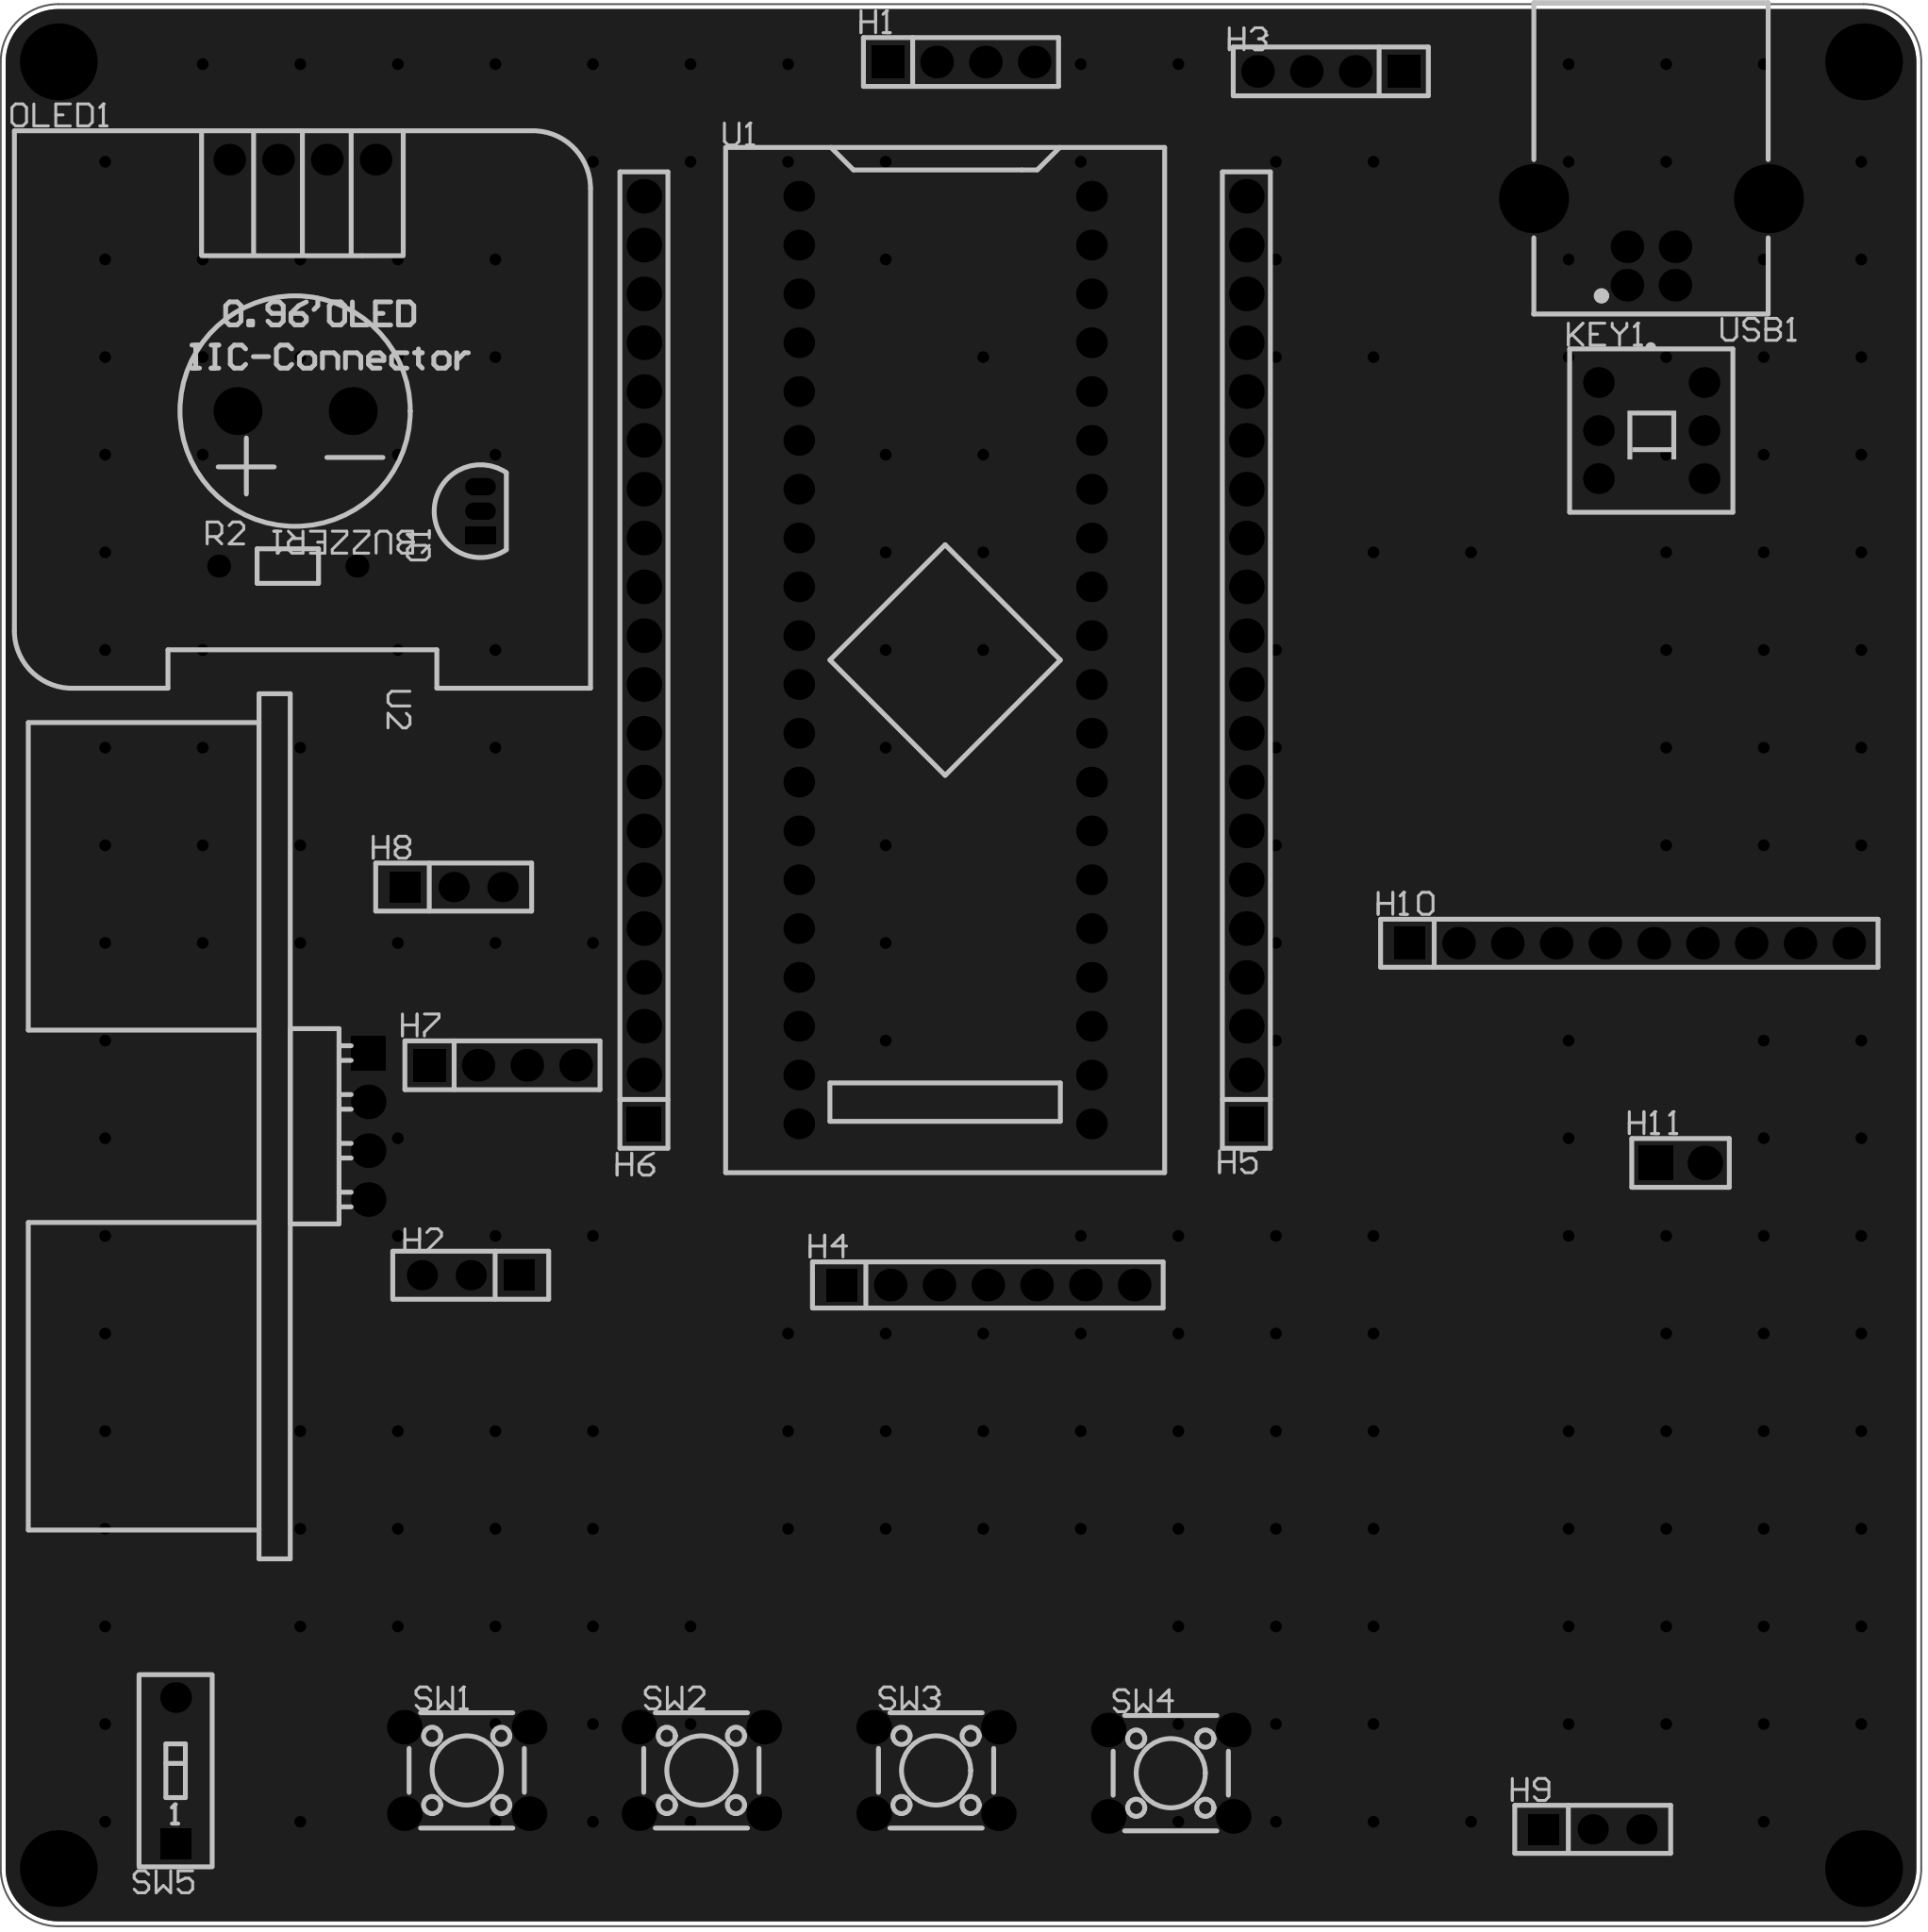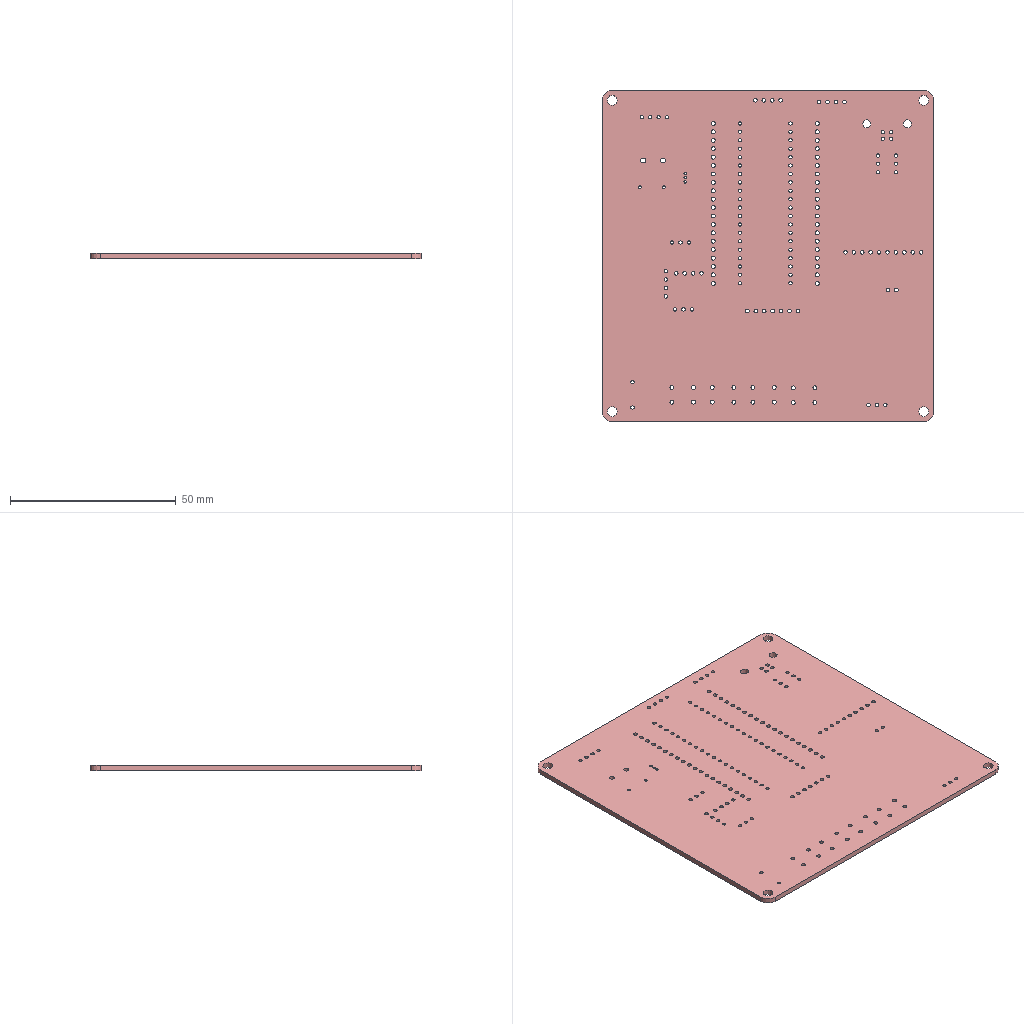Circuit board layout | Altium Designer | box 100 x 100 x 1.6 mm
Layer stack:
# Altium Designer layer stack of  (unit mm; dielectric type: 0 none, 1 core, 2 prepreg, 3 surface material)
index,name,kind,layer,copper_thickness_mm,dielectric_type,dielectric_thickness_mm,dielectric_material,dielectric_constant
0,Top Paste Mask Layer,other,,,,,,
1,Top Silkscreen Layer,other,,,,,,
2,Top Solder Mask Layer,dielectric,,,3,0.01,,3.3
3,Top Layer,copper,Top Layer,0.035,,,,
4,Dielectric1,dielectric,,,3,1.51,FR4,4.5
5,Bottom Layer,copper,Bottom Layer,0.035,,,,
6,Bottom Solder Mask Layer,dielectric,,,3,0.01,,3.3
7,Bottom Silkscreen Layer,other,,,,,,
8,Bottom Paste Mask Layer,other,,,,,,
# drill layer pairs: low layer,high layer
drill_pair,Top Layer,Bottom Layer
Part placement:
Designator,Comment,Layer,Footprint,Center-X(mm),Center-Y(mm),Rotation
BUZZER1,buzzer,TopLayer,BUZ-TH_BD12.0-P6.00-D0.9-RD,95.885,157.734,180
H1,,TopLayer,HDR-TH_4P-P2.54-V-M,130.556,175.895,0
H2,,TopLayer,HDR-TH_3P-P2.54-V-F,105.029,112.776,180
H3,,TopLayer,HDR-TH_4P-P2.54-V-M,149.81,175.405,180
H4,,TopLayer,HDR-TH_7P-P2.54-V-F,131.953,112.268,0
H5,,TopLayer,HDR-TH_20P-P2.54-V-M-1,145.415,144.78,90
H6,,TopLayer,HDR-TH_20P-P2.54-V-M-1,114.046,144.78,90
H7,,TopLayer,HDR-TH_4P-P2.54-V-M,106.68,123.698,0
H8,,TopLayer,HDR-TH_3P-P2.54-V-F,104.14,132.969,0
H9,,TopLayer,HDR-TH_3P-P2.54-V-F,163.449,83.947,0
H10,,TopLayer,HDR-TH_10P-P2.54-V-F,165.354,130.048,0
H11,,TopLayer,HDR-TH_2P-P2.54-V-M-1,168.021,118.618,0
KEY1,Non-latching switch 8.5×8.5, silent,TopLayer,SW-TH_6P-L8.5-W8.5-P2.54,166.497,156.718,270
OLED1,,TopLayer,0.96OLED_4P,96.266,170.815,0
Q1,,TopLayer,S8050_TO_92,105.537,152.527,90
R2,10kΩ,TopLayer,Res_1/8W,95.504,149.669,0
SW5,NDS-01V,TopLayer,SW-TH_2P-L3.9-W9.9-P2.54-LS7.6,89.662,86.995,90
U1,STM32F103C8T6-Card,TopLayer,CONN-TH_L53.3-W22.9_STM32F103C8T6-CARD,129.731,144.78,270
U2,HC-SR04,TopLayer,TH_HC-SR04V,99.695,120.523,270
USB1,,TopLayer,USB__Type-B,166.484,166.533,180
SW1,,TopLayer,SW-TH_4P-L6.0-W6.0-P4.50-LS6.5,104.819,87.011,180
SW2,,TopLayer,SW-TH_4P-L6.0-W6.0-P4.50-LS6.5,117.038,87.011,180
SW3,,TopLayer,SW-TH_4P-L6.0-W6.0-P4.50-LS6.5,129.258,87.011,180
SW4,,TopLayer,SW-TH_4P-L6.0-W6.0-P4.50-LS6.5,141.478,86.868,180
Pad and via stacks:
# Altium Designer via and pad stacks of  (unit mm). Each distinct definition once, with the count of objects using it.
# via: kind,start_layer,end_layer,hole_mm,diameter_mm,mode(0 simple;1 top-mid-bottom;2 full stack),diameter_per_layer,count,example_net
# pad: kind,layer,hole_mm,hole_type(0 round;1 square;2 slot),plating,top_size,top_shape(1 round;2 rect;3 octagon;9 rounded rect),mid_size,bottom_size,mode,footprint,size_per_layer,count,example
pad,Multi-Layer,3,0,plated,4x4,1,4x4,4x4,0,,,4,1
pad,Multi-Layer,1.5,0,plated,2.5x2.5,1,2.5x2.5,2.5x2.5,0,BUZ-TH_BD12.0-P6.00-D0.9-RD,,2,BUZZER1.1
pad,Multi-Layer,1.1,0,plated,1.7x1.7,2,1.7x1.7,1.7x1.7,0,HDR-TH_4P-P2.54-V-M,,3,H1.1
pad,Multi-Layer,1.1,0,plated,1.7x1.7,1,1.7x1.7,1.7x1.7,0,HDR-TH_4P-P2.54-V-M,,9,H1.2
pad,Multi-Layer,1.02,0,plated,1.575x1.575,1,1.575x1.575,1.575x1.575,0,HDR-TH_3P-P2.54-V-F,,6,H2.3
pad,Multi-Layer,1.02,0,plated,1.575x1.575,2,1.575x1.575,1.575x1.575,0,HDR-TH_3P-P2.54-V-F,,3,H2.1
pad,Multi-Layer,1.1,0,plated,1.7x1.7,1,1.7x1.7,1.7x1.7,0,HDR-TH_7P-P2.54-V-F,,6,H4.7
pad,Multi-Layer,1.1,0,plated,1.575x1.7,2,1.575x1.7,1.575x1.7,0,HDR-TH_7P-P2.54-V-F,,1,H4.1
pad,Multi-Layer,1.2,0,plated,1.8x1.8,1,1.8x1.8,1.8x1.8,0,HDR-TH_20P-P2.54-V-M-1,,38,H5.20
pad,Multi-Layer,1.2,0,plated,1.8x1.8,2,1.8x1.8,1.8x1.8,0,HDR-TH_20P-P2.54-V-M-1,,2,H5.1
pad,Multi-Layer,1.1,0,plated,1.7x1.7,1,1.7x1.7,1.7x1.7,0,HDR-TH_10P-P2.54-V-F,,9,H10.10
pad,Multi-Layer,1.1,0,plated,1.575x1.7,2,1.575x1.7,1.575x1.7,0,HDR-TH_10P-P2.54-V-F,,1,H10.1
pad,Multi-Layer,1.1,0,plated,1.8x1.8,1,1.8x1.8,1.8x1.8,0,HDR-TH_2P-P2.54-V-M-1,,1,H11.2
pad,Multi-Layer,1.1,0,plated,1.8x1.8,2,1.8x1.8,1.8x1.8,0,HDR-TH_2P-P2.54-V-M-1,,1,H11.1
pad,Multi-Layer,1,0,plated,1.6x1.6,1,1.6x1.6,1.6x1.6,0,SW-TH_6P-L8.5-W8.5-P2.54,,6,KEY1.4
pad,Multi-Layer,1,0,plated,1.65x1.65,1,1.65x1.65,1.65x1.65,0,0.96OLED_4P,,4,OLED1.4
pad,Multi-Layer,0.701,0,plated,0.8992x1.6,2,0.8992x1.6,0.8992x1.6,0,S8050_TO_92,,1,Q1.1
pad,Multi-Layer,0.701,0,plated,0.8992x1.6,1,0.8992x1.6,0.8992x1.6,0,S8050_TO_92,,2,Q1.2
pad,Multi-Layer,0.8001,0,plated,1.199x1.199,1,1.199x1.199,1.199x1.199,0,Res_1/8W,,2,R2.1
pad,Multi-Layer,1,0,plated,1.6x1.6,2,1.6x1.6,1.6x1.6,0,SW-TH_2P-L3.9-W9.9-P2.54-LS7.6,,1,SW5.1
pad,Multi-Layer,1,0,plated,1.6x1.6,1,1.6x1.6,1.6x1.6,0,SW-TH_2P-L3.9-W9.9-P2.54-LS7.6,,1,SW5.2
pad,Multi-Layer,1,0,plated,1.6x1.6,1,1.6x1.6,1.6x1.6,0,CONN-TH_L53.3-W22.9_STM32F103C8T6-CARD,,40,U1.1
pad,Multi-Layer,1.001,0,plated,1.8x1.8,1,1.8x1.8,1.8x1.8,0,TH_HC-SR04V,,3,U2.4
pad,Multi-Layer,1.001,0,plated,1.8x1.8,2,1.8x1.8,1.8x1.8,0,TH_HC-SR04V,,1,U2.1
pad,Multi-Layer,1.1,0,plated,1.7x1.7,1,1.7x1.7,1.7x1.7,0,USB_ Type-B,,4,USB1.3
pad,Multi-Layer,2.4,0,plated,3.6x3.6,1,3.6x3.6,3.6x3.6,0,USB_ Type-B,,2,USB1.5
pad,Multi-Layer,1.2,0,plated,1.8x1.8,1,1.8x1.8,1.8x1.8,0,SW-TH_4P-L6.0-W6.0-P4.50-LS6.5,,16,SW1.1
via,Top Layer,Bottom Layer,0.3048,0.61,0,,197,GND
Copper pours:
name,layer,net,type(0 solid;1 hatched;2 none)
Bottom Layer-GND,Bottom Layer,GND,0
Top Layer-GND,Top Layer,GND,0
Design rules, without the lines most boards share:
# Altium Designer design rules of  (exported by Altium Designer, unit mm)
# columns: name | kind | enabled | priority | scope1 | scope2 | descriptor | typed fields (field=value)
copperThickness1oz_2 | 2 | enabled | 2 | All | All | Width Constraint (Min=5mil) (Max=100mil) (Preferred=30mil) (All) |
viaSize | 11 | enabled | 1 | All | All | Routing Via (MinHoleWidth=11.811mil) (MaxHoleWidth=248.032mil) (PreferredHoleWidth=12.008mil) (MinWidth=19.685mil) (MaxWidth=393.701mil) (PreferedWidth=24.016mil) (All) | via_min_hole=0.3 via_max_hole=6.3 via_preferred_diameter=0.61 via_preferred_hole=0.305
solderMaskExpansion | 13 | enabled | 2 | All | All | Solder Mask Expansion (Expansion =2.008mil) (All) | expansion=0.051